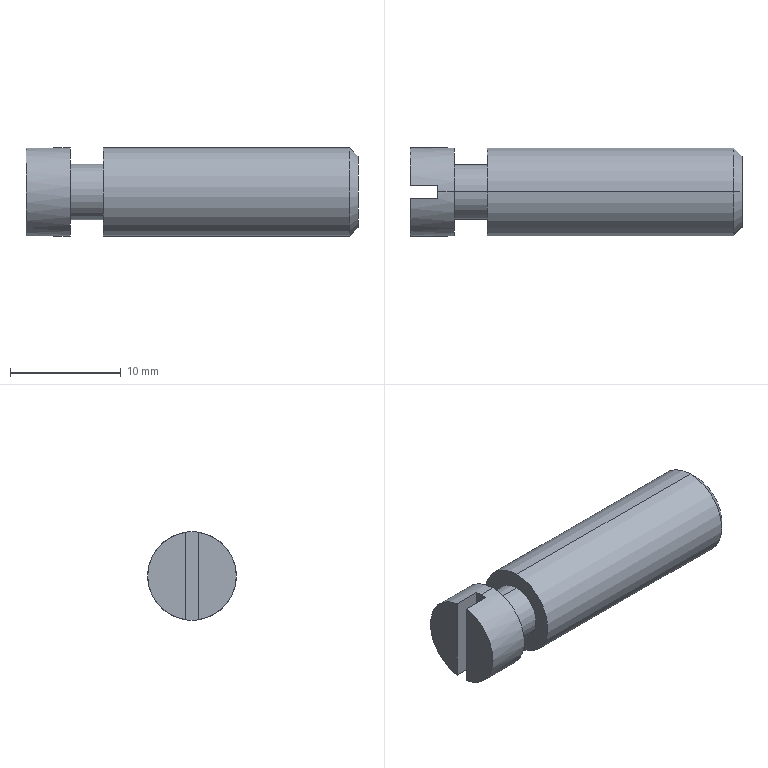Part | STEP file | 0217_Z_SBSP8-30-1 | 1 solid | 16 faces | box 30 x 8 x 8 mm | volume 1385 mm3 | plane 8 | cylinder 6 | cone 2 | commonest cylinder face diameters 8 x4 5 x2
STEP:
#1=CARTESIAN_POINT('',(0.,0.,0.));
#2=DIRECTION('',(0.,0.,1.));
#3=DIRECTION('',(1.,0.,0.));
#4=AXIS2_PLACEMENT_3D('',#1,#2,#3);
#5=CARTESIAN_POINT('',(7.,0.,-4.));
#6=VERTEX_POINT('',#5);
#7=CARTESIAN_POINT('',(7.,0.,4.));
#8=VERTEX_POINT('',#7);
#9=CARTESIAN_POINT('',(7.,0.,0.));
#10=DIRECTION('',(1.,0.,0.));
#11=DIRECTION('',(0.,0.,-1.));
#12=AXIS2_PLACEMENT_3D('',#9,#10,#11);
#13=CIRCLE('',#12,4.);
#14=CARTESIAN_POINT('',(14.617,0.,0.));
#15=DIRECTION('',(1.,0.,0.));
#16=DIRECTION('',(0.,0.,-1.));
#17=AXIS2_PLACEMENT_3D('',#14,#15,#16);
#18=CYLINDRICAL_SURFACE('',#17,4.);
#19=CARTESIAN_POINT('',(0.,-7.617));
#20=DIRECTION('',(1.,0.));
#21=VECTOR('',#20,1.);
#22=LINE('',#19,#21);
#23=(GEOMETRIC_REPRESENTATION_CONTEXT(2)PARAMETRIC_REPRESENTATION_CONTEXT()REPRESENTATION_CONTEXT('',''));
#24=DEFINITIONAL_REPRESENTATION('',(#22),#23);
#25=PCURVE('',#18,#24);
#26=CARTESIAN_POINT('',(7.,4.,0.));
#27=DIRECTION('',(1.,0.,0.));
#28=DIRECTION('',(0.,0.,-1.));
#29=AXIS2_PLACEMENT_3D('',#26,#27,#28);
#30=PLANE('',#29);
#31=CARTESIAN_POINT('',(0.,-4.));
#32=DIRECTION('',(1.,0.));
#33=AXIS2_PLACEMENT_2D('',#31,#32);
#34=CIRCLE('',#33,4.);
#35=(GEOMETRIC_REPRESENTATION_CONTEXT(2)PARAMETRIC_REPRESENTATION_CONTEXT()REPRESENTATION_CONTEXT('',''));
#36=DEFINITIONAL_REPRESENTATION('',(#34),#35);
#37=PCURVE('',#30,#36);
#38=SURFACE_CURVE('',#13,(#25,#37),.PCURVE_S1.);
#39=EDGE_CURVE('',#6,#8,#38,.T.);
#40=ORIENTED_EDGE('',*,*,#39,.T.);
#41=CARTESIAN_POINT('',(29.233,0.,4.));
#42=VERTEX_POINT('',#41);
#43=CARTESIAN_POINT('',(14.617,0.,4.));
#44=DIRECTION('',(1.,0.,0.));
#45=VECTOR('',#44,1.);
#46=LINE('',#43,#45);
#47=CARTESIAN_POINT('',(3.142,0.));
#48=DIRECTION('',(0.,1.));
#49=VECTOR('',#48,1.);
#50=LINE('',#47,#49);
#51=(GEOMETRIC_REPRESENTATION_CONTEXT(2)PARAMETRIC_REPRESENTATION_CONTEXT()REPRESENTATION_CONTEXT('',''));
#52=DEFINITIONAL_REPRESENTATION('',(#50),#51);
#53=PCURVE('',#18,#52);
#54=CARTESIAN_POINT('',(14.617,0.,0.));
#55=DIRECTION('',(1.,0.,0.));
#56=DIRECTION('',(0.,0.,-1.));
#57=AXIS2_PLACEMENT_3D('',#54,#55,#56);
#58=CYLINDRICAL_SURFACE('',#57,4.);
#59=CARTESIAN_POINT('',(3.142,0.));
#60=DIRECTION('',(0.,1.));
#61=VECTOR('',#60,1.);
#62=LINE('',#59,#61);
#63=(GEOMETRIC_REPRESENTATION_CONTEXT(2)PARAMETRIC_REPRESENTATION_CONTEXT()REPRESENTATION_CONTEXT('',''));
#64=DEFINITIONAL_REPRESENTATION('',(#62),#63);
#65=PCURVE('',#58,#64);
#66=SURFACE_CURVE('',#46,(#53,#65),.PCURVE_S1.);
#67=EDGE_CURVE('',#8,#42,#66,.T.);
#68=ORIENTED_EDGE('',*,*,#67,.T.);
#69=CARTESIAN_POINT('',(29.233,0.,-4.));
#70=VERTEX_POINT('',#69);
#71=CARTESIAN_POINT('',(29.233,0.,0.));
#72=DIRECTION('',(-1.,0.,0.));
#73=DIRECTION('',(0.,0.,-1.));
#74=AXIS2_PLACEMENT_3D('',#71,#72,#73);
#75=CIRCLE('',#74,4.);
#76=CARTESIAN_POINT('',(6.283,14.617));
#77=DIRECTION('',(-1.,0.));
#78=VECTOR('',#77,1.);
#79=LINE('',#76,#78);
#80=(GEOMETRIC_REPRESENTATION_CONTEXT(2)PARAMETRIC_REPRESENTATION_CONTEXT()REPRESENTATION_CONTEXT('',''));
#81=DEFINITIONAL_REPRESENTATION('',(#79),#80);
#82=PCURVE('',#18,#81);
#83=CARTESIAN_POINT('',(29.233,0.,0.));
#84=DIRECTION('',(-1.,0.,0.));
#85=DIRECTION('',(0.,0.,1.));
#86=AXIS2_PLACEMENT_3D('',#83,#84,#85);
#87=CONICAL_SURFACE('',#86,4.,0.7854);
#88=CARTESIAN_POINT('',(-3.142,0.));
#89=DIRECTION('',(1.,0.));
#90=VECTOR('',#89,1.);
#91=LINE('',#88,#90);
#92=(GEOMETRIC_REPRESENTATION_CONTEXT(2)PARAMETRIC_REPRESENTATION_CONTEXT()REPRESENTATION_CONTEXT('',''));
#93=DEFINITIONAL_REPRESENTATION('',(#91),#92);
#94=PCURVE('',#87,#93);
#95=SURFACE_CURVE('',#75,(#82,#94),.PCURVE_S1.);
#96=EDGE_CURVE('',#42,#70,#95,.T.);
#97=ORIENTED_EDGE('',*,*,#96,.T.);
#98=CARTESIAN_POINT('',(14.617,0.,-4.));
#99=DIRECTION('',(1.,0.,0.));
#100=VECTOR('',#99,1.);
#101=LINE('',#98,#100);
#102=CARTESIAN_POINT('',(0.,0.));
#103=DIRECTION('',(0.,1.));
#104=VECTOR('',#103,1.);
#105=LINE('',#102,#104);
#106=(GEOMETRIC_REPRESENTATION_CONTEXT(2)PARAMETRIC_REPRESENTATION_CONTEXT()REPRESENTATION_CONTEXT('',''));
#107=DEFINITIONAL_REPRESENTATION('',(#105),#106);
#108=PCURVE('',#18,#107);
#109=CARTESIAN_POINT('',(6.283,0.));
#110=DIRECTION('',(0.,1.));
#111=VECTOR('',#110,1.);
#112=LINE('',#109,#111);
#113=(GEOMETRIC_REPRESENTATION_CONTEXT(2)PARAMETRIC_REPRESENTATION_CONTEXT()REPRESENTATION_CONTEXT('',''));
#114=DEFINITIONAL_REPRESENTATION('',(#112),#113);
#115=PCURVE('',#58,#114);
#116=SURFACE_CURVE('',#101,(#108,#115),.PCURVE_S1.);
#117=EDGE_CURVE('',#6,#70,#116,.T.);
#118=ORIENTED_EDGE('',*,*,#117,.F.);
#119=EDGE_LOOP('',(#40,#68,#97,#118));
#120=FACE_BOUND('',#119,.T.);
#121=ADVANCED_FACE('',(#120),#18,.T.);
#122=CARTESIAN_POINT('',(30.,0.,3.233));
#123=VERTEX_POINT('',#122);
#124=CARTESIAN_POINT('',(30.,0.,-3.233));
#125=VERTEX_POINT('',#124);
#126=CARTESIAN_POINT('',(30.,0.,0.));
#127=DIRECTION('',(-1.,0.,0.));
#128=DIRECTION('',(0.,0.,1.));
#129=AXIS2_PLACEMENT_3D('',#126,#127,#128);
#130=CIRCLE('',#129,3.233);
#131=CARTESIAN_POINT('',(0.,-0.767));
#132=DIRECTION('',(1.,0.));
#133=VECTOR('',#132,1.);
#134=LINE('',#131,#133);
#135=(GEOMETRIC_REPRESENTATION_CONTEXT(2)PARAMETRIC_REPRESENTATION_CONTEXT()REPRESENTATION_CONTEXT('',''));
#136=DEFINITIONAL_REPRESENTATION('',(#134),#135);
#137=PCURVE('',#87,#136);
#138=CARTESIAN_POINT('',(30.,1.617,0.));
#139=DIRECTION('',(1.,0.,0.));
#140=DIRECTION('',(0.,0.,-1.));
#141=AXIS2_PLACEMENT_3D('',#138,#139,#140);
#142=PLANE('',#141);
#143=CARTESIAN_POINT('',(-3.233,-1.617));
#144=CARTESIAN_POINT('',(-3.233,3.983));
#145=CARTESIAN_POINT('',(1.616,1.183));
#146=CARTESIAN_POINT('',(6.466,-1.617));
#147=CARTESIAN_POINT('',(1.616,-4.416));
#148=CARTESIAN_POINT('',(-3.233,-7.216));
#149=CARTESIAN_POINT('',(-3.233,-1.617));
#150=(BOUNDED_CURVE()B_SPLINE_CURVE(2,(#143,#144,#145,#146,#147,#148,#149),.UNSPECIFIED.,.T.,.F.)B_SPLINE_CURVE_WITH_KNOTS((1,2,2,2,2,1),(-2.094,0.,2.094,4.189,6.283,8.378),.UNSPECIFIED.)CURVE()GEOMETRIC_REPRESENTATION_ITEM()RATIONAL_B_SPLINE_CURVE((1.,0.5,1.,0.5,1.,0.5,1.))REPRESENTATION_ITEM(''));
#151=(GEOMETRIC_REPRESENTATION_CONTEXT(2)PARAMETRIC_REPRESENTATION_CONTEXT()REPRESENTATION_CONTEXT('',''));
#152=DEFINITIONAL_REPRESENTATION('',(#150),#151);
#153=PCURVE('',#142,#152);
#154=SURFACE_CURVE('',#130,(#137,#153),.PCURVE_S1.);
#155=EDGE_CURVE('',#123,#125,#154,.T.);
#156=ORIENTED_EDGE('',*,*,#155,.T.);
#157=CARTESIAN_POINT('',(29.233,0.,-4.));
#158=DIRECTION('',(-0.7071,0.,-0.7071));
#159=VECTOR('',#158,1.);
#160=LINE('',#157,#159);
#161=CARTESIAN_POINT('',(3.142,0.));
#162=DIRECTION('',(0.,1.));
#163=VECTOR('',#162,1.);
#164=LINE('',#161,#163);
#165=(GEOMETRIC_REPRESENTATION_CONTEXT(2)PARAMETRIC_REPRESENTATION_CONTEXT()REPRESENTATION_CONTEXT('',''));
#166=DEFINITIONAL_REPRESENTATION('',(#164),#165);
#167=PCURVE('',#87,#166);
#168=CARTESIAN_POINT('',(29.233,0.,0.));
#169=DIRECTION('',(-1.,0.,0.));
#170=DIRECTION('',(0.,0.,1.));
#171=AXIS2_PLACEMENT_3D('',#168,#169,#170);
#172=CONICAL_SURFACE('',#171,4.,0.7854);
#173=CARTESIAN_POINT('',(3.142,0.));
#174=DIRECTION('',(0.,1.));
#175=VECTOR('',#174,1.);
#176=LINE('',#173,#175);
#177=(GEOMETRIC_REPRESENTATION_CONTEXT(2)PARAMETRIC_REPRESENTATION_CONTEXT()REPRESENTATION_CONTEXT('',''));
#178=DEFINITIONAL_REPRESENTATION('',(#176),#177);
#179=PCURVE('',#172,#178);
#180=SURFACE_CURVE('',#160,(#167,#179),.PCURVE_S1.);
#181=EDGE_CURVE('',#125,#70,#180,.T.);
#182=ORIENTED_EDGE('',*,*,#181,.T.);
#183=ORIENTED_EDGE('',*,*,#96,.F.);
#184=CARTESIAN_POINT('',(29.233,0.,4.));
#185=DIRECTION('',(-0.7071,0.,0.7071));
#186=VECTOR('',#185,1.);
#187=LINE('',#184,#186);
#188=CARTESIAN_POINT('',(0.,0.));
#189=DIRECTION('',(0.,1.));
#190=VECTOR('',#189,1.);
#191=LINE('',#188,#190);
#192=(GEOMETRIC_REPRESENTATION_CONTEXT(2)PARAMETRIC_REPRESENTATION_CONTEXT()REPRESENTATION_CONTEXT('',''));
#193=DEFINITIONAL_REPRESENTATION('',(#191),#192);
#194=PCURVE('',#87,#193);
#195=CARTESIAN_POINT('',(6.283,0.));
#196=DIRECTION('',(0.,1.));
#197=VECTOR('',#196,1.);
#198=LINE('',#195,#197);
#199=(GEOMETRIC_REPRESENTATION_CONTEXT(2)PARAMETRIC_REPRESENTATION_CONTEXT()REPRESENTATION_CONTEXT('',''));
#200=DEFINITIONAL_REPRESENTATION('',(#198),#199);
#201=PCURVE('',#172,#200);
#202=SURFACE_CURVE('',#187,(#194,#201),.PCURVE_S1.);
#203=EDGE_CURVE('',#123,#42,#202,.T.);
#204=ORIENTED_EDGE('',*,*,#203,.F.);
#205=EDGE_LOOP('',(#156,#182,#183,#204));
#206=FACE_BOUND('',#205,.T.);
#207=ADVANCED_FACE('',(#206),#87,.T.);
#208=CARTESIAN_POINT('',(4.,0.,-2.5));
#209=VERTEX_POINT('',#208);
#210=CARTESIAN_POINT('',(4.,0.,2.5));
#211=VERTEX_POINT('',#210);
#212=CARTESIAN_POINT('',(4.,0.,0.));
#213=DIRECTION('',(1.,0.,0.));
#214=DIRECTION('',(0.,0.,-1.));
#215=AXIS2_PLACEMENT_3D('',#212,#213,#214);
#216=CIRCLE('',#215,2.5);
#217=CARTESIAN_POINT('',(5.5,0.,0.));
#218=DIRECTION('',(1.,0.,0.));
#219=DIRECTION('',(0.,0.,-1.));
#220=AXIS2_PLACEMENT_3D('',#217,#218,#219);
#221=CYLINDRICAL_SURFACE('',#220,2.5);
#222=CARTESIAN_POINT('',(0.,-1.5));
#223=DIRECTION('',(1.,0.));
#224=VECTOR('',#223,1.);
#225=LINE('',#222,#224);
#226=(GEOMETRIC_REPRESENTATION_CONTEXT(2)PARAMETRIC_REPRESENTATION_CONTEXT()REPRESENTATION_CONTEXT('',''));
#227=DEFINITIONAL_REPRESENTATION('',(#225),#226);
#228=PCURVE('',#221,#227);
#229=CARTESIAN_POINT('',(4.,4.,0.));
#230=DIRECTION('',(-1.,0.,0.));
#231=DIRECTION('',(0.,0.,1.));
#232=AXIS2_PLACEMENT_3D('',#229,#230,#231);
#233=PLANE('',#232);
#234=CARTESIAN_POINT('',(-2.5,-4.));
#235=CARTESIAN_POINT('',(-2.5,0.3301));
#236=CARTESIAN_POINT('',(1.25,-1.835));
#237=CARTESIAN_POINT('',(5.,-4.));
#238=CARTESIAN_POINT('',(1.25,-6.165));
#239=CARTESIAN_POINT('',(-2.5,-8.33));
#240=CARTESIAN_POINT('',(-2.5,-4.));
#241=(BOUNDED_CURVE()B_SPLINE_CURVE(2,(#234,#235,#236,#237,#238,#239,#240),.UNSPECIFIED.,.T.,.F.)B_SPLINE_CURVE_WITH_KNOTS((1,2,2,2,2,1),(-2.094,0.,2.094,4.189,6.283,8.378),.UNSPECIFIED.)CURVE()GEOMETRIC_REPRESENTATION_ITEM()RATIONAL_B_SPLINE_CURVE((1.,0.5,1.,0.5,1.,0.5,1.))REPRESENTATION_ITEM(''));
#242=(GEOMETRIC_REPRESENTATION_CONTEXT(2)PARAMETRIC_REPRESENTATION_CONTEXT()REPRESENTATION_CONTEXT('',''));
#243=DEFINITIONAL_REPRESENTATION('',(#241),#242);
#244=PCURVE('',#233,#243);
#245=SURFACE_CURVE('',#216,(#228,#244),.PCURVE_S1.);
#246=EDGE_CURVE('',#209,#211,#245,.T.);
#247=ORIENTED_EDGE('',*,*,#246,.T.);
#248=CARTESIAN_POINT('',(7.,0.,2.5));
#249=VERTEX_POINT('',#248);
#250=CARTESIAN_POINT('',(5.5,0.,2.5));
#251=DIRECTION('',(1.,0.,0.));
#252=VECTOR('',#251,1.);
#253=LINE('',#250,#252);
#254=CARTESIAN_POINT('',(3.142,0.));
#255=DIRECTION('',(0.,1.));
#256=VECTOR('',#255,1.);
#257=LINE('',#254,#256);
#258=(GEOMETRIC_REPRESENTATION_CONTEXT(2)PARAMETRIC_REPRESENTATION_CONTEXT()REPRESENTATION_CONTEXT('',''));
#259=DEFINITIONAL_REPRESENTATION('',(#257),#258);
#260=PCURVE('',#221,#259);
#261=CARTESIAN_POINT('',(5.5,0.,0.));
#262=DIRECTION('',(1.,0.,0.));
#263=DIRECTION('',(0.,0.,-1.));
#264=AXIS2_PLACEMENT_3D('',#261,#262,#263);
#265=CYLINDRICAL_SURFACE('',#264,2.5);
#266=CARTESIAN_POINT('',(3.142,0.));
#267=DIRECTION('',(0.,1.));
#268=VECTOR('',#267,1.);
#269=LINE('',#266,#268);
#270=(GEOMETRIC_REPRESENTATION_CONTEXT(2)PARAMETRIC_REPRESENTATION_CONTEXT()REPRESENTATION_CONTEXT('',''));
#271=DEFINITIONAL_REPRESENTATION('',(#269),#270);
#272=PCURVE('',#265,#271);
#273=SURFACE_CURVE('',#253,(#260,#272),.PCURVE_S1.);
#274=EDGE_CURVE('',#211,#249,#273,.T.);
#275=ORIENTED_EDGE('',*,*,#274,.T.);
#276=CARTESIAN_POINT('',(7.,0.,-2.5));
#277=VERTEX_POINT('',#276);
#278=CARTESIAN_POINT('',(7.,0.,0.));
#279=DIRECTION('',(-1.,0.,0.));
#280=DIRECTION('',(0.,0.,-1.));
#281=AXIS2_PLACEMENT_3D('',#278,#279,#280);
#282=CIRCLE('',#281,2.5);
#283=CARTESIAN_POINT('',(6.283,1.5));
#284=DIRECTION('',(-1.,0.));
#285=VECTOR('',#284,1.);
#286=LINE('',#283,#285);
#287=(GEOMETRIC_REPRESENTATION_CONTEXT(2)PARAMETRIC_REPRESENTATION_CONTEXT()REPRESENTATION_CONTEXT('',''));
#288=DEFINITIONAL_REPRESENTATION('',(#286),#287);
#289=PCURVE('',#221,#288);
#290=CARTESIAN_POINT('',(2.5,-4.));
#291=CARTESIAN_POINT('',(2.5,-8.33));
#292=CARTESIAN_POINT('',(-1.25,-6.165));
#293=CARTESIAN_POINT('',(-5.,-4.));
#294=CARTESIAN_POINT('',(-1.25,-1.835));
#295=CARTESIAN_POINT('',(2.5,0.3301));
#296=CARTESIAN_POINT('',(2.5,-4.));
#297=(BOUNDED_CURVE()B_SPLINE_CURVE(2,(#290,#291,#292,#293,#294,#295,#296),.UNSPECIFIED.,.T.,.F.)B_SPLINE_CURVE_WITH_KNOTS((1,2,2,2,2,1),(-2.094,0.,2.094,4.189,6.283,8.378),.UNSPECIFIED.)CURVE()GEOMETRIC_REPRESENTATION_ITEM()RATIONAL_B_SPLINE_CURVE((1.,0.5,1.,0.5,1.,0.5,1.))REPRESENTATION_ITEM(''));
#298=(GEOMETRIC_REPRESENTATION_CONTEXT(2)PARAMETRIC_REPRESENTATION_CONTEXT()REPRESENTATION_CONTEXT('',''));
#299=DEFINITIONAL_REPRESENTATION('',(#297),#298);
#300=PCURVE('',#30,#299);
#301=SURFACE_CURVE('',#282,(#289,#300),.PCURVE_S1.);
#302=EDGE_CURVE('',#249,#277,#301,.T.);
#303=ORIENTED_EDGE('',*,*,#302,.T.);
#304=CARTESIAN_POINT('',(5.5,0.,-2.5));
#305=DIRECTION('',(1.,0.,0.));
#306=VECTOR('',#305,1.);
#307=LINE('',#304,#306);
#308=CARTESIAN_POINT('',(0.,0.));
#309=DIRECTION('',(0.,1.));
#310=VECTOR('',#309,1.);
#311=LINE('',#308,#310);
#312=(GEOMETRIC_REPRESENTATION_CONTEXT(2)PARAMETRIC_REPRESENTATION_CONTEXT()REPRESENTATION_CONTEXT('',''));
#313=DEFINITIONAL_REPRESENTATION('',(#311),#312);
#314=PCURVE('',#221,#313);
#315=CARTESIAN_POINT('',(6.283,0.));
#316=DIRECTION('',(0.,1.));
#317=VECTOR('',#316,1.);
#318=LINE('',#315,#317);
#319=(GEOMETRIC_REPRESENTATION_CONTEXT(2)PARAMETRIC_REPRESENTATION_CONTEXT()REPRESENTATION_CONTEXT('',''));
#320=DEFINITIONAL_REPRESENTATION('',(#318),#319);
#321=PCURVE('',#265,#320);
#322=SURFACE_CURVE('',#307,(#314,#321),.PCURVE_S1.);
#323=EDGE_CURVE('',#209,#277,#322,.T.);
#324=ORIENTED_EDGE('',*,*,#323,.F.);
#325=EDGE_LOOP('',(#247,#275,#303,#324));
#326=FACE_BOUND('',#325,.T.);
#327=ADVANCED_FACE('',(#326),#221,.T.);
#328=CARTESIAN_POINT('',(2.5,0.6,3.955));
#329=VERTEX_POINT('',#328);
#330=CARTESIAN_POINT('',(2.5,0.,4.));
#331=VERTEX_POINT('',#330);
#332=CARTESIAN_POINT('',(2.5,0.,0.));
#333=DIRECTION('',(1.,0.,0.));
#334=DIRECTION('',(0.,0.,-1.));
#335=AXIS2_PLACEMENT_3D('',#332,#333,#334);
#336=CIRCLE('',#335,4.);
#337=CARTESIAN_POINT('',(14.617,0.,0.));
#338=DIRECTION('',(1.,0.,0.));
#339=DIRECTION('',(0.,0.,-1.));
#340=AXIS2_PLACEMENT_3D('',#337,#338,#339);
#341=CYLINDRICAL_SURFACE('',#340,4.);
#342=CARTESIAN_POINT('',(0.,-12.117));
#343=DIRECTION('',(1.,0.));
#344=VECTOR('',#343,1.);
#345=LINE('',#342,#344);
#346=(GEOMETRIC_REPRESENTATION_CONTEXT(2)PARAMETRIC_REPRESENTATION_CONTEXT()REPRESENTATION_CONTEXT('',''));
#347=DEFINITIONAL_REPRESENTATION('',(#345),#346);
#348=PCURVE('',#341,#347);
#349=CARTESIAN_POINT('',(2.5,-0.6,4.));
#350=DIRECTION('',(1.,0.,0.));
#351=DIRECTION('',(0.,0.,-1.));
#352=AXIS2_PLACEMENT_3D('',#349,#350,#351);
#353=PLANE('',#352);
#354=CARTESIAN_POINT('',(4.,0.6));
#355=DIRECTION('',(1.,0.));
#356=AXIS2_PLACEMENT_2D('',#354,#355);
#357=CIRCLE('',#356,4.);
#358=(GEOMETRIC_REPRESENTATION_CONTEXT(2)PARAMETRIC_REPRESENTATION_CONTEXT()REPRESENTATION_CONTEXT('',''));
#359=DEFINITIONAL_REPRESENTATION('',(#357),#358);
#360=PCURVE('',#353,#359);
#361=SURFACE_CURVE('',#336,(#348,#360),.PCURVE_S1.);
#362=EDGE_CURVE('',#329,#331,#361,.T.);
#363=ORIENTED_EDGE('',*,*,#362,.T.);
#364=CARTESIAN_POINT('',(4.,0.,4.));
#365=VERTEX_POINT('',#364);
#366=CARTESIAN_POINT('',(14.617,0.,4.));
#367=DIRECTION('',(1.,0.,0.));
#368=VECTOR('',#367,1.);
#369=LINE('',#366,#368);
#370=CARTESIAN_POINT('',(3.142,0.));
#371=DIRECTION('',(0.,1.));
#372=VECTOR('',#371,1.);
#373=LINE('',#370,#372);
#374=(GEOMETRIC_REPRESENTATION_CONTEXT(2)PARAMETRIC_REPRESENTATION_CONTEXT()REPRESENTATION_CONTEXT('',''));
#375=DEFINITIONAL_REPRESENTATION('',(#373),#374);
#376=PCURVE('',#341,#375);
#377=CARTESIAN_POINT('',(14.617,0.,0.));
#378=DIRECTION('',(1.,0.,0.));
#379=DIRECTION('',(0.,0.,-1.));
#380=AXIS2_PLACEMENT_3D('',#377,#378,#379);
#381=CYLINDRICAL_SURFACE('',#380,4.);
#382=CARTESIAN_POINT('',(3.142,0.));
#383=DIRECTION('',(0.,1.));
#384=VECTOR('',#383,1.);
#385=LINE('',#382,#384);
#386=(GEOMETRIC_REPRESENTATION_CONTEXT(2)PARAMETRIC_REPRESENTATION_CONTEXT()REPRESENTATION_CONTEXT('',''));
#387=DEFINITIONAL_REPRESENTATION('',(#385),#386);
#388=PCURVE('',#381,#387);
#389=SURFACE_CURVE('',#369,(#376,#388),.PCURVE_S1.);
#390=EDGE_CURVE('',#331,#365,#389,.T.);
#391=ORIENTED_EDGE('',*,*,#390,.T.);
#392=CARTESIAN_POINT('',(4.,0.,-4.));
#393=VERTEX_POINT('',#392);
#394=CARTESIAN_POINT('',(4.,0.,0.));
#395=DIRECTION('',(-1.,0.,0.));
#396=DIRECTION('',(0.,0.,-1.));
#397=AXIS2_PLACEMENT_3D('',#394,#395,#396);
#398=CIRCLE('',#397,4.);
#399=CARTESIAN_POINT('',(6.283,-10.617));
#400=DIRECTION('',(-1.,0.));
#401=VECTOR('',#400,1.);
#402=LINE('',#399,#401);
#403=(GEOMETRIC_REPRESENTATION_CONTEXT(2)PARAMETRIC_REPRESENTATION_CONTEXT()REPRESENTATION_CONTEXT('',''));
#404=DEFINITIONAL_REPRESENTATION('',(#402),#403);
#405=PCURVE('',#341,#404);
#406=CARTESIAN_POINT('',(0.,-4.));
#407=DIRECTION('',(-1.,0.));
#408=AXIS2_PLACEMENT_2D('',#406,#407);
#409=CIRCLE('',#408,4.);
#410=(GEOMETRIC_REPRESENTATION_CONTEXT(2)PARAMETRIC_REPRESENTATION_CONTEXT()REPRESENTATION_CONTEXT('',''));
#411=DEFINITIONAL_REPRESENTATION('',(#409),#410);
#412=PCURVE('',#233,#411);
#413=SURFACE_CURVE('',#398,(#405,#412),.PCURVE_S1.);
#414=EDGE_CURVE('',#365,#393,#413,.T.);
#415=ORIENTED_EDGE('',*,*,#414,.T.);
#416=CARTESIAN_POINT('',(2.5,0.,-4.));
#417=VERTEX_POINT('',#416);
#418=CARTESIAN_POINT('',(14.617,0.,-4.));
#419=DIRECTION('',(1.,0.,0.));
#420=VECTOR('',#419,1.);
#421=LINE('',#418,#420);
#422=CARTESIAN_POINT('',(0.,0.));
#423=DIRECTION('',(0.,1.));
#424=VECTOR('',#423,1.);
#425=LINE('',#422,#424);
#426=(GEOMETRIC_REPRESENTATION_CONTEXT(2)PARAMETRIC_REPRESENTATION_CONTEXT()REPRESENTATION_CONTEXT('',''));
#427=DEFINITIONAL_REPRESENTATION('',(#425),#426);
#428=PCURVE('',#341,#427);
#429=CARTESIAN_POINT('',(6.283,0.));
#430=DIRECTION('',(0.,1.));
#431=VECTOR('',#430,1.);
#432=LINE('',#429,#431);
#433=(GEOMETRIC_REPRESENTATION_CONTEXT(2)PARAMETRIC_REPRESENTATION_CONTEXT()REPRESENTATION_CONTEXT('',''));
#434=DEFINITIONAL_REPRESENTATION('',(#432),#433);
#435=PCURVE('',#381,#434);
#436=SURFACE_CURVE('',#421,(#428,#435),.PCURVE_S1.);
#437=EDGE_CURVE('',#417,#393,#436,.T.);
#438=ORIENTED_EDGE('',*,*,#437,.F.);
#439=CARTESIAN_POINT('',(2.5,0.6,-3.955));
#440=VERTEX_POINT('',#439);
#441=CARTESIAN_POINT('',(2.5,0.,0.));
#442=DIRECTION('',(1.,0.,0.));
#443=DIRECTION('',(0.,0.,-1.));
#444=AXIS2_PLACEMENT_3D('',#441,#442,#443);
#445=CIRCLE('',#444,4.);
#446=CARTESIAN_POINT('',(0.,-12.117));
#447=DIRECTION('',(1.,0.));
#448=VECTOR('',#447,1.);
#449=LINE('',#446,#448);
#450=(GEOMETRIC_REPRESENTATION_CONTEXT(2)PARAMETRIC_REPRESENTATION_CONTEXT()REPRESENTATION_CONTEXT('',''));
#451=DEFINITIONAL_REPRESENTATION('',(#449),#450);
#452=PCURVE('',#341,#451);
#453=CARTESIAN_POINT('',(4.,0.6));
#454=DIRECTION('',(1.,0.));
#455=AXIS2_PLACEMENT_2D('',#453,#454);
#456=CIRCLE('',#455,4.);
#457=(GEOMETRIC_REPRESENTATION_CONTEXT(2)PARAMETRIC_REPRESENTATION_CONTEXT()REPRESENTATION_CONTEXT('',''));
#458=DEFINITIONAL_REPRESENTATION('',(#456),#457);
#459=PCURVE('',#353,#458);
#460=SURFACE_CURVE('',#445,(#452,#459),.PCURVE_S1.);
#461=EDGE_CURVE('',#417,#440,#460,.T.);
#462=ORIENTED_EDGE('',*,*,#461,.T.);
#463=CARTESIAN_POINT('',(0.,0.6,-3.955));
#464=VERTEX_POINT('',#463);
#465=CARTESIAN_POINT('',(14.617,0.6,-3.955));
#466=DIRECTION('',(-1.,0.,0.));
#467=VECTOR('',#466,1.);
#468=LINE('',#465,#467);
#469=CARTESIAN_POINT('',(0.1506,0.));
#470=DIRECTION('',(0.,-1.));
#471=VECTOR('',#470,1.);
#472=LINE('',#469,#471);
#473=(GEOMETRIC_REPRESENTATION_CONTEXT(2)PARAMETRIC_REPRESENTATION_CONTEXT()REPRESENTATION_CONTEXT('',''));
#474=DEFINITIONAL_REPRESENTATION('',(#472),#473);
#475=PCURVE('',#341,#474);
#476=CARTESIAN_POINT('',(2.5,0.6,4.));
#477=DIRECTION('',(0.,1.,0.));
#478=DIRECTION('',(0.,0.,1.));
#479=AXIS2_PLACEMENT_3D('',#476,#477,#478);
#480=PLANE('',#479);
#481=CARTESIAN_POINT('',(-7.955,12.117));
#482=DIRECTION('',(0.,-1.));
#483=VECTOR('',#482,1.);
#484=LINE('',#481,#483);
#485=(GEOMETRIC_REPRESENTATION_CONTEXT(2)PARAMETRIC_REPRESENTATION_CONTEXT()REPRESENTATION_CONTEXT('',''));
#486=DEFINITIONAL_REPRESENTATION('',(#484),#485);
#487=PCURVE('',#480,#486);
#488=SURFACE_CURVE('',#468,(#475,#487),.PCURVE_S1.);
#489=EDGE_CURVE('',#440,#464,#488,.T.);
#490=ORIENTED_EDGE('',*,*,#489,.T.);
#491=CARTESIAN_POINT('',(0.,0.6,3.955));
#492=VERTEX_POINT('',#491);
#493=CARTESIAN_POINT('',(0.,0.,0.));
#494=DIRECTION('',(1.,0.,0.));
#495=DIRECTION('',(0.,0.,-1.));
#496=AXIS2_PLACEMENT_3D('',#493,#494,#495);
#497=CIRCLE('',#496,4.);
#498=CARTESIAN_POINT('',(0.,-14.617));
#499=DIRECTION('',(1.,0.));
#500=VECTOR('',#499,1.);
#501=LINE('',#498,#500);
#502=(GEOMETRIC_REPRESENTATION_CONTEXT(2)PARAMETRIC_REPRESENTATION_CONTEXT()REPRESENTATION_CONTEXT('',''));
#503=DEFINITIONAL_REPRESENTATION('',(#501),#502);
#504=PCURVE('',#341,#503);
#505=CARTESIAN_POINT('',(0.,2.,0.));
#506=DIRECTION('',(-1.,0.,0.));
#507=DIRECTION('',(0.,0.,1.));
#508=AXIS2_PLACEMENT_3D('',#505,#506,#507);
#509=PLANE('',#508);
#510=CARTESIAN_POINT('',(-4.,-2.));
#511=CARTESIAN_POINT('',(-4.,4.928));
#512=CARTESIAN_POINT('',(2.,1.464));
#513=CARTESIAN_POINT('',(8.,-2.));
#514=CARTESIAN_POINT('',(2.,-5.464));
#515=CARTESIAN_POINT('',(-4.,-8.928));
#516=CARTESIAN_POINT('',(-4.,-2.));
#517=(BOUNDED_CURVE()B_SPLINE_CURVE(2,(#510,#511,#512,#513,#514,#515,#516),.UNSPECIFIED.,.T.,.F.)B_SPLINE_CURVE_WITH_KNOTS((1,2,2,2,2,1),(-2.094,0.,2.094,4.189,6.283,8.378),.UNSPECIFIED.)CURVE()GEOMETRIC_REPRESENTATION_ITEM()RATIONAL_B_SPLINE_CURVE((1.,0.5,1.,0.5,1.,0.5,1.))REPRESENTATION_ITEM(''));
#518=(GEOMETRIC_REPRESENTATION_CONTEXT(2)PARAMETRIC_REPRESENTATION_CONTEXT()REPRESENTATION_CONTEXT('',''));
#519=DEFINITIONAL_REPRESENTATION('',(#517),#518);
#520=PCURVE('',#509,#519);
#521=SURFACE_CURVE('',#497,(#504,#520),.PCURVE_S1.);
#522=EDGE_CURVE('',#464,#492,#521,.T.);
#523=ORIENTED_EDGE('',*,*,#522,.T.);
#524=CARTESIAN_POINT('',(14.617,0.6,3.955));
#525=DIRECTION('',(1.,0.,0.));
#526=VECTOR('',#525,1.);
#527=LINE('',#524,#526);
#528=CARTESIAN_POINT('',(2.991,0.));
#529=DIRECTION('',(0.,1.));
#530=VECTOR('',#529,1.);
#531=LINE('',#528,#530);
#532=(GEOMETRIC_REPRESENTATION_CONTEXT(2)PARAMETRIC_REPRESENTATION_CONTEXT()REPRESENTATION_CONTEXT('',''));
#533=DEFINITIONAL_REPRESENTATION('',(#531),#532);
#534=PCURVE('',#341,#533);
#535=CARTESIAN_POINT('',(-0.04526,12.117));
#536=DIRECTION('',(0.,1.));
#537=VECTOR('',#536,1.);
#538=LINE('',#535,#537);
#539=(GEOMETRIC_REPRESENTATION_CONTEXT(2)PARAMETRIC_REPRESENTATION_CONTEXT()REPRESENTATION_CONTEXT('',''));
#540=DEFINITIONAL_REPRESENTATION('',(#538),#539);
#541=PCURVE('',#480,#540);
#542=SURFACE_CURVE('',#527,(#534,#541),.PCURVE_S1.);
#543=EDGE_CURVE('',#492,#329,#542,.T.);
#544=ORIENTED_EDGE('',*,*,#543,.T.);
#545=EDGE_LOOP('',(#363,#391,#415,#438,#462,#490,#523,#544));
#546=FACE_BOUND('',#545,.T.);
#547=ADVANCED_FACE('',(#546),#341,.T.);
#548=ORIENTED_EDGE('',*,*,#67,.F.);
#549=CARTESIAN_POINT('',(7.,0.,0.));
#550=DIRECTION('',(1.,0.,0.));
#551=DIRECTION('',(0.,0.,-1.));
#552=AXIS2_PLACEMENT_3D('',#549,#550,#551);
#553=CIRCLE('',#552,4.);
#554=CARTESIAN_POINT('',(0.,-7.617));
#555=DIRECTION('',(1.,0.));
#556=VECTOR('',#555,1.);
#557=LINE('',#554,#556);
#558=(GEOMETRIC_REPRESENTATION_CONTEXT(2)PARAMETRIC_REPRESENTATION_CONTEXT()REPRESENTATION_CONTEXT('',''));
#559=DEFINITIONAL_REPRESENTATION('',(#557),#558);
#560=PCURVE('',#58,#559);
#561=CARTESIAN_POINT('',(0.,-4.));
#562=DIRECTION('',(1.,0.));
#563=AXIS2_PLACEMENT_2D('',#561,#562);
#564=CIRCLE('',#563,4.);
#565=(GEOMETRIC_REPRESENTATION_CONTEXT(2)PARAMETRIC_REPRESENTATION_CONTEXT()REPRESENTATION_CONTEXT('',''));
#566=DEFINITIONAL_REPRESENTATION('',(#564),#565);
#567=PCURVE('',#30,#566);
#568=SURFACE_CURVE('',#553,(#560,#567),.PCURVE_S1.);
#569=EDGE_CURVE('',#8,#6,#568,.T.);
#570=ORIENTED_EDGE('',*,*,#569,.T.);
#571=ORIENTED_EDGE('',*,*,#117,.T.);
#572=CARTESIAN_POINT('',(29.233,0.,0.));
#573=DIRECTION('',(-1.,0.,0.));
#574=DIRECTION('',(0.,0.,-1.));
#575=AXIS2_PLACEMENT_3D('',#572,#573,#574);
#576=CIRCLE('',#575,4.);
#577=CARTESIAN_POINT('',(6.283,14.617));
#578=DIRECTION('',(-1.,0.));
#579=VECTOR('',#578,1.);
#580=LINE('',#577,#579);
#581=(GEOMETRIC_REPRESENTATION_CONTEXT(2)PARAMETRIC_REPRESENTATION_CONTEXT()REPRESENTATION_CONTEXT('',''));
#582=DEFINITIONAL_REPRESENTATION('',(#580),#581);
#583=PCURVE('',#58,#582);
#584=CARTESIAN_POINT('',(3.142,0.));
#585=DIRECTION('',(1.,0.));
#586=VECTOR('',#585,1.);
#587=LINE('',#584,#586);
#588=(GEOMETRIC_REPRESENTATION_CONTEXT(2)PARAMETRIC_REPRESENTATION_CONTEXT()REPRESENTATION_CONTEXT('',''));
#589=DEFINITIONAL_REPRESENTATION('',(#587),#588);
#590=PCURVE('',#172,#589);
#591=SURFACE_CURVE('',#576,(#583,#590),.PCURVE_S1.);
#592=EDGE_CURVE('',#70,#42,#591,.T.);
#593=ORIENTED_EDGE('',*,*,#592,.T.);
#594=EDGE_LOOP('',(#548,#570,#571,#593));
#595=FACE_BOUND('',#594,.T.);
#596=ADVANCED_FACE('',(#595),#58,.T.);
#597=CARTESIAN_POINT('',(7.,0.,0.));
#598=DIRECTION('',(-1.,0.,0.));
#599=DIRECTION('',(0.,0.,-1.));
#600=AXIS2_PLACEMENT_3D('',#597,#598,#599);
#601=CIRCLE('',#600,2.5);
#602=CARTESIAN_POINT('',(2.5,-4.));
#603=CARTESIAN_POINT('',(2.5,-8.33));
#604=CARTESIAN_POINT('',(-1.25,-6.165));
#605=CARTESIAN_POINT('',(-5.,-4.));
#606=CARTESIAN_POINT('',(-1.25,-1.835));
#607=CARTESIAN_POINT('',(2.5,0.3301));
#608=CARTESIAN_POINT('',(2.5,-4.));
#609=(BOUNDED_CURVE()B_SPLINE_CURVE(2,(#602,#603,#604,#605,#606,#607,#608),.UNSPECIFIED.,.T.,.F.)B_SPLINE_CURVE_WITH_KNOTS((1,2,2,2,2,1),(-2.094,0.,2.094,4.189,6.283,8.378),.UNSPECIFIED.)CURVE()GEOMETRIC_REPRESENTATION_ITEM()RATIONAL_B_SPLINE_CURVE((1.,0.5,1.,0.5,1.,0.5,1.))REPRESENTATION_ITEM(''));
#610=(GEOMETRIC_REPRESENTATION_CONTEXT(2)PARAMETRIC_REPRESENTATION_CONTEXT()REPRESENTATION_CONTEXT('',''));
#611=DEFINITIONAL_REPRESENTATION('',(#609),#610);
#612=PCURVE('',#30,#611);
#613=CARTESIAN_POINT('',(6.283,1.5));
#614=DIRECTION('',(-1.,0.));
#615=VECTOR('',#614,1.);
#616=LINE('',#613,#615);
#617=(GEOMETRIC_REPRESENTATION_CONTEXT(2)PARAMETRIC_REPRESENTATION_CONTEXT()REPRESENTATION_CONTEXT('',''));
#618=DEFINITIONAL_REPRESENTATION('',(#616),#617);
#619=PCURVE('',#265,#618);
#620=SURFACE_CURVE('',#601,(#612,#619),.PCURVE_S1.);
#621=EDGE_CURVE('',#277,#249,#620,.T.);
#622=ORIENTED_EDGE('',*,*,#621,.F.);
#623=ORIENTED_EDGE('',*,*,#302,.F.);
#624=EDGE_LOOP('',(#622,#623));
#625=FACE_BOUND('',#624,.T.);
#626=ORIENTED_EDGE('',*,*,#39,.F.);
#627=ORIENTED_EDGE('',*,*,#569,.F.);
#628=EDGE_LOOP('',(#626,#627));
#629=FACE_BOUND('',#628,.T.);
#630=ADVANCED_FACE('',(#625,#629),#30,.F.);
#631=ORIENTED_EDGE('',*,*,#181,.F.);
#632=CARTESIAN_POINT('',(30.,0.,0.));
#633=DIRECTION('',(-1.,0.,0.));
#634=DIRECTION('',(0.,0.,1.));
#635=AXIS2_PLACEMENT_3D('',#632,#633,#634);
#636=CIRCLE('',#635,3.233);
#637=CARTESIAN_POINT('',(0.,-0.767));
#638=DIRECTION('',(1.,0.));
#639=VECTOR('',#638,1.);
#640=LINE('',#637,#639);
#641=(GEOMETRIC_REPRESENTATION_CONTEXT(2)PARAMETRIC_REPRESENTATION_CONTEXT()REPRESENTATION_CONTEXT('',''));
#642=DEFINITIONAL_REPRESENTATION('',(#640),#641);
#643=PCURVE('',#172,#642);
#644=CARTESIAN_POINT('',(-3.233,-1.617));
#645=CARTESIAN_POINT('',(-3.233,3.983));
#646=CARTESIAN_POINT('',(1.616,1.183));
#647=CARTESIAN_POINT('',(6.466,-1.617));
#648=CARTESIAN_POINT('',(1.616,-4.416));
#649=CARTESIAN_POINT('',(-3.233,-7.216));
#650=CARTESIAN_POINT('',(-3.233,-1.617));
#651=(BOUNDED_CURVE()B_SPLINE_CURVE(2,(#644,#645,#646,#647,#648,#649,#650),.UNSPECIFIED.,.T.,.F.)B_SPLINE_CURVE_WITH_KNOTS((1,2,2,2,2,1),(-2.094,0.,2.094,4.189,6.283,8.378),.UNSPECIFIED.)CURVE()GEOMETRIC_REPRESENTATION_ITEM()RATIONAL_B_SPLINE_CURVE((1.,0.5,1.,0.5,1.,0.5,1.))REPRESENTATION_ITEM(''));
#652=(GEOMETRIC_REPRESENTATION_CONTEXT(2)PARAMETRIC_REPRESENTATION_CONTEXT()REPRESENTATION_CONTEXT('',''));
#653=DEFINITIONAL_REPRESENTATION('',(#651),#652);
#654=PCURVE('',#142,#653);
#655=SURFACE_CURVE('',#636,(#643,#654),.PCURVE_S1.);
#656=EDGE_CURVE('',#125,#123,#655,.T.);
#657=ORIENTED_EDGE('',*,*,#656,.T.);
#658=ORIENTED_EDGE('',*,*,#203,.T.);
#659=ORIENTED_EDGE('',*,*,#592,.F.);
#660=EDGE_LOOP('',(#631,#657,#658,#659));
#661=FACE_BOUND('',#660,.T.);
#662=ADVANCED_FACE('',(#661),#172,.T.);
#663=ORIENTED_EDGE('',*,*,#274,.F.);
#664=CARTESIAN_POINT('',(4.,0.,0.));
#665=DIRECTION('',(1.,0.,0.));
#666=DIRECTION('',(0.,0.,-1.));
#667=AXIS2_PLACEMENT_3D('',#664,#665,#666);
#668=CIRCLE('',#667,2.5);
#669=CARTESIAN_POINT('',(0.,-1.5));
#670=DIRECTION('',(1.,0.));
#671=VECTOR('',#670,1.);
#672=LINE('',#669,#671);
#673=(GEOMETRIC_REPRESENTATION_CONTEXT(2)PARAMETRIC_REPRESENTATION_CONTEXT()REPRESENTATION_CONTEXT('',''));
#674=DEFINITIONAL_REPRESENTATION('',(#672),#673);
#675=PCURVE('',#265,#674);
#676=CARTESIAN_POINT('',(-2.5,-4.));
#677=CARTESIAN_POINT('',(-2.5,0.3301));
#678=CARTESIAN_POINT('',(1.25,-1.835));
#679=CARTESIAN_POINT('',(5.,-4.));
#680=CARTESIAN_POINT('',(1.25,-6.165));
#681=CARTESIAN_POINT('',(-2.5,-8.33));
#682=CARTESIAN_POINT('',(-2.5,-4.));
#683=(BOUNDED_CURVE()B_SPLINE_CURVE(2,(#676,#677,#678,#679,#680,#681,#682),.UNSPECIFIED.,.T.,.F.)B_SPLINE_CURVE_WITH_KNOTS((1,2,2,2,2,1),(-2.094,0.,2.094,4.189,6.283,8.378),.UNSPECIFIED.)CURVE()GEOMETRIC_REPRESENTATION_ITEM()RATIONAL_B_SPLINE_CURVE((1.,0.5,1.,0.5,1.,0.5,1.))REPRESENTATION_ITEM(''));
#684=(GEOMETRIC_REPRESENTATION_CONTEXT(2)PARAMETRIC_REPRESENTATION_CONTEXT()REPRESENTATION_CONTEXT('',''));
#685=DEFINITIONAL_REPRESENTATION('',(#683),#684);
#686=PCURVE('',#233,#685);
#687=SURFACE_CURVE('',#668,(#675,#686),.PCURVE_S1.);
#688=EDGE_CURVE('',#211,#209,#687,.T.);
#689=ORIENTED_EDGE('',*,*,#688,.T.);
#690=ORIENTED_EDGE('',*,*,#323,.T.);
#691=ORIENTED_EDGE('',*,*,#621,.T.);
#692=EDGE_LOOP('',(#663,#689,#690,#691));
#693=FACE_BOUND('',#692,.T.);
#694=ADVANCED_FACE('',(#693),#265,.T.);
#695=ORIENTED_EDGE('',*,*,#155,.F.);
#696=ORIENTED_EDGE('',*,*,#656,.F.);
#697=EDGE_LOOP('',(#695,#696));
#698=FACE_BOUND('',#697,.T.);
#699=ADVANCED_FACE('',(#698),#142,.T.);
#700=ORIENTED_EDGE('',*,*,#246,.F.);
#701=ORIENTED_EDGE('',*,*,#688,.F.);
#702=EDGE_LOOP('',(#700,#701));
#703=FACE_BOUND('',#702,.T.);
#704=CARTESIAN_POINT('',(4.,0.,0.));
#705=DIRECTION('',(-1.,0.,0.));
#706=DIRECTION('',(0.,0.,-1.));
#707=AXIS2_PLACEMENT_3D('',#704,#705,#706);
#708=CIRCLE('',#707,4.);
#709=CARTESIAN_POINT('',(0.,-4.));
#710=DIRECTION('',(-1.,0.));
#711=AXIS2_PLACEMENT_2D('',#709,#710);
#712=CIRCLE('',#711,4.);
#713=(GEOMETRIC_REPRESENTATION_CONTEXT(2)PARAMETRIC_REPRESENTATION_CONTEXT()REPRESENTATION_CONTEXT('',''));
#714=DEFINITIONAL_REPRESENTATION('',(#712),#713);
#715=PCURVE('',#233,#714);
#716=CARTESIAN_POINT('',(6.283,-10.617));
#717=DIRECTION('',(-1.,0.));
#718=VECTOR('',#717,1.);
#719=LINE('',#716,#718);
#720=(GEOMETRIC_REPRESENTATION_CONTEXT(2)PARAMETRIC_REPRESENTATION_CONTEXT()REPRESENTATION_CONTEXT('',''));
#721=DEFINITIONAL_REPRESENTATION('',(#719),#720);
#722=PCURVE('',#381,#721);
#723=SURFACE_CURVE('',#708,(#715,#722),.PCURVE_S1.);
#724=EDGE_CURVE('',#393,#365,#723,.T.);
#725=ORIENTED_EDGE('',*,*,#724,.F.);
#726=ORIENTED_EDGE('',*,*,#414,.F.);
#727=EDGE_LOOP('',(#725,#726));
#728=FACE_BOUND('',#727,.T.);
#729=ADVANCED_FACE('',(#703,#728),#233,.F.);
#730=ORIENTED_EDGE('',*,*,#390,.F.);
#731=CARTESIAN_POINT('',(2.5,-0.6,3.955));
#732=VERTEX_POINT('',#731);
#733=CARTESIAN_POINT('',(2.5,0.,0.));
#734=DIRECTION('',(1.,0.,0.));
#735=DIRECTION('',(0.,0.,-1.));
#736=AXIS2_PLACEMENT_3D('',#733,#734,#735);
#737=CIRCLE('',#736,4.);
#738=CARTESIAN_POINT('',(0.,-12.117));
#739=DIRECTION('',(1.,0.));
#740=VECTOR('',#739,1.);
#741=LINE('',#738,#740);
#742=(GEOMETRIC_REPRESENTATION_CONTEXT(2)PARAMETRIC_REPRESENTATION_CONTEXT()REPRESENTATION_CONTEXT('',''));
#743=DEFINITIONAL_REPRESENTATION('',(#741),#742);
#744=PCURVE('',#381,#743);
#745=CARTESIAN_POINT('',(4.,0.6));
#746=DIRECTION('',(1.,0.));
#747=AXIS2_PLACEMENT_2D('',#745,#746);
#748=CIRCLE('',#747,4.);
#749=(GEOMETRIC_REPRESENTATION_CONTEXT(2)PARAMETRIC_REPRESENTATION_CONTEXT()REPRESENTATION_CONTEXT('',''));
#750=DEFINITIONAL_REPRESENTATION('',(#748),#749);
#751=PCURVE('',#353,#750);
#752=SURFACE_CURVE('',#737,(#744,#751),.PCURVE_S1.);
#753=EDGE_CURVE('',#331,#732,#752,.T.);
#754=ORIENTED_EDGE('',*,*,#753,.T.);
#755=CARTESIAN_POINT('',(0.,-0.6,3.955));
#756=VERTEX_POINT('',#755);
#757=CARTESIAN_POINT('',(14.617,-0.6,3.955));
#758=DIRECTION('',(-1.,0.,0.));
#759=VECTOR('',#758,1.);
#760=LINE('',#757,#759);
#761=CARTESIAN_POINT('',(3.292,0.));
#762=DIRECTION('',(0.,-1.));
#763=VECTOR('',#762,1.);
#764=LINE('',#761,#763);
#765=(GEOMETRIC_REPRESENTATION_CONTEXT(2)PARAMETRIC_REPRESENTATION_CONTEXT()REPRESENTATION_CONTEXT('',''));
#766=DEFINITIONAL_REPRESENTATION('',(#764),#765);
#767=PCURVE('',#381,#766);
#768=CARTESIAN_POINT('',(0.,-0.6,4.));
#769=DIRECTION('',(0.,-1.,0.));
#770=DIRECTION('',(0.,0.,-1.));
#771=AXIS2_PLACEMENT_3D('',#768,#769,#770);
#772=PLANE('',#771);
#773=CARTESIAN_POINT('',(0.04526,14.617));
#774=DIRECTION('',(0.,-1.));
#775=VECTOR('',#774,1.);
#776=LINE('',#773,#775);
#777=(GEOMETRIC_REPRESENTATION_CONTEXT(2)PARAMETRIC_REPRESENTATION_CONTEXT()REPRESENTATION_CONTEXT('',''));
#778=DEFINITIONAL_REPRESENTATION('',(#776),#777);
#779=PCURVE('',#772,#778);
#780=SURFACE_CURVE('',#760,(#767,#779),.PCURVE_S1.);
#781=EDGE_CURVE('',#732,#756,#780,.T.);
#782=ORIENTED_EDGE('',*,*,#781,.T.);
#783=CARTESIAN_POINT('',(0.,-0.6,-3.955));
#784=VERTEX_POINT('',#783);
#785=CARTESIAN_POINT('',(0.,0.,0.));
#786=DIRECTION('',(1.,0.,0.));
#787=DIRECTION('',(0.,0.,-1.));
#788=AXIS2_PLACEMENT_3D('',#785,#786,#787);
#789=CIRCLE('',#788,4.);
#790=CARTESIAN_POINT('',(0.,-14.617));
#791=DIRECTION('',(1.,0.));
#792=VECTOR('',#791,1.);
#793=LINE('',#790,#792);
#794=(GEOMETRIC_REPRESENTATION_CONTEXT(2)PARAMETRIC_REPRESENTATION_CONTEXT()REPRESENTATION_CONTEXT('',''));
#795=DEFINITIONAL_REPRESENTATION('',(#793),#794);
#796=PCURVE('',#381,#795);
#797=CARTESIAN_POINT('',(0.,2.,0.));
#798=DIRECTION('',(-1.,0.,0.));
#799=DIRECTION('',(0.,0.,1.));
#800=AXIS2_PLACEMENT_3D('',#797,#798,#799);
#801=PLANE('',#800);
#802=CARTESIAN_POINT('',(-4.,-2.));
#803=CARTESIAN_POINT('',(-4.,4.928));
#804=CARTESIAN_POINT('',(2.,1.464));
#805=CARTESIAN_POINT('',(8.,-2.));
#806=CARTESIAN_POINT('',(2.,-5.464));
#807=CARTESIAN_POINT('',(-4.,-8.928));
#808=CARTESIAN_POINT('',(-4.,-2.));
#809=(BOUNDED_CURVE()B_SPLINE_CURVE(2,(#802,#803,#804,#805,#806,#807,#808),.UNSPECIFIED.,.T.,.F.)B_SPLINE_CURVE_WITH_KNOTS((1,2,2,2,2,1),(-2.094,0.,2.094,4.189,6.283,8.378),.UNSPECIFIED.)CURVE()GEOMETRIC_REPRESENTATION_ITEM()RATIONAL_B_SPLINE_CURVE((1.,0.5,1.,0.5,1.,0.5,1.))REPRESENTATION_ITEM(''));
#810=(GEOMETRIC_REPRESENTATION_CONTEXT(2)PARAMETRIC_REPRESENTATION_CONTEXT()REPRESENTATION_CONTEXT('',''));
#811=DEFINITIONAL_REPRESENTATION('',(#809),#810);
#812=PCURVE('',#801,#811);
#813=SURFACE_CURVE('',#789,(#796,#812),.PCURVE_S1.);
#814=EDGE_CURVE('',#756,#784,#813,.T.);
#815=ORIENTED_EDGE('',*,*,#814,.T.);
#816=CARTESIAN_POINT('',(2.5,-0.6,-3.955));
#817=VERTEX_POINT('',#816);
#818=CARTESIAN_POINT('',(14.617,-0.6,-3.955));
#819=DIRECTION('',(1.,0.,0.));
#820=VECTOR('',#819,1.);
#821=LINE('',#818,#820);
#822=CARTESIAN_POINT('',(6.133,0.));
#823=DIRECTION('',(0.,1.));
#824=VECTOR('',#823,1.);
#825=LINE('',#822,#824);
#826=(GEOMETRIC_REPRESENTATION_CONTEXT(2)PARAMETRIC_REPRESENTATION_CONTEXT()REPRESENTATION_CONTEXT('',''));
#827=DEFINITIONAL_REPRESENTATION('',(#825),#826);
#828=PCURVE('',#381,#827);
#829=CARTESIAN_POINT('',(7.955,14.617));
#830=DIRECTION('',(0.,1.));
#831=VECTOR('',#830,1.);
#832=LINE('',#829,#831);
#833=(GEOMETRIC_REPRESENTATION_CONTEXT(2)PARAMETRIC_REPRESENTATION_CONTEXT()REPRESENTATION_CONTEXT('',''));
#834=DEFINITIONAL_REPRESENTATION('',(#832),#833);
#835=PCURVE('',#772,#834);
#836=SURFACE_CURVE('',#821,(#828,#835),.PCURVE_S1.);
#837=EDGE_CURVE('',#784,#817,#836,.T.);
#838=ORIENTED_EDGE('',*,*,#837,.T.);
#839=CARTESIAN_POINT('',(2.5,0.,0.));
#840=DIRECTION('',(1.,0.,0.));
#841=DIRECTION('',(0.,0.,-1.));
#842=AXIS2_PLACEMENT_3D('',#839,#840,#841);
#843=CIRCLE('',#842,4.);
#844=CARTESIAN_POINT('',(0.,-12.117));
#845=DIRECTION('',(1.,0.));
#846=VECTOR('',#845,1.);
#847=LINE('',#844,#846);
#848=(GEOMETRIC_REPRESENTATION_CONTEXT(2)PARAMETRIC_REPRESENTATION_CONTEXT()REPRESENTATION_CONTEXT('',''));
#849=DEFINITIONAL_REPRESENTATION('',(#847),#848);
#850=PCURVE('',#381,#849);
#851=CARTESIAN_POINT('',(4.,0.6));
#852=DIRECTION('',(1.,0.));
#853=AXIS2_PLACEMENT_2D('',#851,#852);
#854=CIRCLE('',#853,4.);
#855=(GEOMETRIC_REPRESENTATION_CONTEXT(2)PARAMETRIC_REPRESENTATION_CONTEXT()REPRESENTATION_CONTEXT('',''));
#856=DEFINITIONAL_REPRESENTATION('',(#854),#855);
#857=PCURVE('',#353,#856);
#858=SURFACE_CURVE('',#843,(#850,#857),.PCURVE_S1.);
#859=EDGE_CURVE('',#817,#417,#858,.T.);
#860=ORIENTED_EDGE('',*,*,#859,.T.);
#861=ORIENTED_EDGE('',*,*,#437,.T.);
#862=ORIENTED_EDGE('',*,*,#724,.T.);
#863=EDGE_LOOP('',(#730,#754,#782,#815,#838,#860,#861,#862));
#864=FACE_BOUND('',#863,.T.);
#865=ADVANCED_FACE('',(#864),#381,.T.);
#866=CARTESIAN_POINT('',(0.,-0.6,0.));
#867=DIRECTION('',(0.,0.,-1.));
#868=VECTOR('',#867,1.);
#869=LINE('',#866,#868);
#870=CARTESIAN_POINT('',(0.,-2.6));
#871=DIRECTION('',(-1.,0.));
#872=VECTOR('',#871,1.);
#873=LINE('',#870,#872);
#874=(GEOMETRIC_REPRESENTATION_CONTEXT(2)PARAMETRIC_REPRESENTATION_CONTEXT()REPRESENTATION_CONTEXT('',''));
#875=DEFINITIONAL_REPRESENTATION('',(#873),#874);
#876=PCURVE('',#801,#875);
#877=CARTESIAN_POINT('',(4.,0.));
#878=DIRECTION('',(1.,0.));
#879=VECTOR('',#878,1.);
#880=LINE('',#877,#879);
#881=(GEOMETRIC_REPRESENTATION_CONTEXT(2)PARAMETRIC_REPRESENTATION_CONTEXT()REPRESENTATION_CONTEXT('',''));
#882=DEFINITIONAL_REPRESENTATION('',(#880),#881);
#883=PCURVE('',#772,#882);
#884=SURFACE_CURVE('',#869,(#876,#883),.PCURVE_S1.);
#885=EDGE_CURVE('',#756,#784,#884,.T.);
#886=ORIENTED_EDGE('',*,*,#885,.T.);
#887=ORIENTED_EDGE('',*,*,#814,.F.);
#888=EDGE_LOOP('',(#886,#887));
#889=FACE_BOUND('',#888,.T.);
#890=ADVANCED_FACE('',(#889),#801,.T.);
#891=ORIENTED_EDGE('',*,*,#885,.F.);
#892=ORIENTED_EDGE('',*,*,#781,.F.);
#893=CARTESIAN_POINT('',(2.5,-0.6,4.));
#894=DIRECTION('',(0.,0.,1.));
#895=VECTOR('',#894,1.);
#896=LINE('',#893,#895);
#897=CARTESIAN_POINT('',(0.,2.5));
#898=DIRECTION('',(-1.,0.));
#899=VECTOR('',#898,1.);
#900=LINE('',#897,#899);
#901=(GEOMETRIC_REPRESENTATION_CONTEXT(2)PARAMETRIC_REPRESENTATION_CONTEXT()REPRESENTATION_CONTEXT('',''));
#902=DEFINITIONAL_REPRESENTATION('',(#900),#901);
#903=PCURVE('',#772,#902);
#904=CARTESIAN_POINT('',(0.,0.));
#905=DIRECTION('',(-1.,0.));
#906=VECTOR('',#905,1.);
#907=LINE('',#904,#906);
#908=(GEOMETRIC_REPRESENTATION_CONTEXT(2)PARAMETRIC_REPRESENTATION_CONTEXT()REPRESENTATION_CONTEXT('',''));
#909=DEFINITIONAL_REPRESENTATION('',(#907),#908);
#910=PCURVE('',#353,#909);
#911=SURFACE_CURVE('',#896,(#903,#910),.PCURVE_S1.);
#912=EDGE_CURVE('',#817,#732,#911,.T.);
#913=ORIENTED_EDGE('',*,*,#912,.F.);
#914=ORIENTED_EDGE('',*,*,#837,.F.);
#915=EDGE_LOOP('',(#891,#892,#913,#914));
#916=FACE_BOUND('',#915,.T.);
#917=ADVANCED_FACE('',(#916),#772,.F.);
#918=CARTESIAN_POINT('',(2.5,0.6,4.));
#919=DIRECTION('',(0.,0.,-1.));
#920=VECTOR('',#919,1.);
#921=LINE('',#918,#920);
#922=CARTESIAN_POINT('',(0.,0.));
#923=DIRECTION('',(-1.,0.));
#924=VECTOR('',#923,1.);
#925=LINE('',#922,#924);
#926=(GEOMETRIC_REPRESENTATION_CONTEXT(2)PARAMETRIC_REPRESENTATION_CONTEXT()REPRESENTATION_CONTEXT('',''));
#927=DEFINITIONAL_REPRESENTATION('',(#925),#926);
#928=PCURVE('',#480,#927);
#929=CARTESIAN_POINT('',(0.,1.2));
#930=DIRECTION('',(1.,0.));
#931=VECTOR('',#930,1.);
#932=LINE('',#929,#931);
#933=(GEOMETRIC_REPRESENTATION_CONTEXT(2)PARAMETRIC_REPRESENTATION_CONTEXT()REPRESENTATION_CONTEXT('',''));
#934=DEFINITIONAL_REPRESENTATION('',(#932),#933);
#935=PCURVE('',#353,#934);
#936=SURFACE_CURVE('',#921,(#928,#935),.PCURVE_S1.);
#937=EDGE_CURVE('',#329,#440,#936,.T.);
#938=ORIENTED_EDGE('',*,*,#937,.F.);
#939=ORIENTED_EDGE('',*,*,#543,.F.);
#940=CARTESIAN_POINT('',(0.,0.6,4.));
#941=DIRECTION('',(0.,0.,1.));
#942=VECTOR('',#941,1.);
#943=LINE('',#940,#942);
#944=CARTESIAN_POINT('',(0.,-2.5));
#945=DIRECTION('',(1.,0.));
#946=VECTOR('',#945,1.);
#947=LINE('',#944,#946);
#948=(GEOMETRIC_REPRESENTATION_CONTEXT(2)PARAMETRIC_REPRESENTATION_CONTEXT()REPRESENTATION_CONTEXT('',''));
#949=DEFINITIONAL_REPRESENTATION('',(#947),#948);
#950=PCURVE('',#480,#949);
#951=CARTESIAN_POINT('',(4.,-1.4));
#952=DIRECTION('',(1.,0.));
#953=VECTOR('',#952,1.);
#954=LINE('',#951,#953);
#955=(GEOMETRIC_REPRESENTATION_CONTEXT(2)PARAMETRIC_REPRESENTATION_CONTEXT()REPRESENTATION_CONTEXT('',''));
#956=DEFINITIONAL_REPRESENTATION('',(#954),#955);
#957=PCURVE('',#509,#956);
#958=SURFACE_CURVE('',#943,(#950,#957),.PCURVE_S1.);
#959=EDGE_CURVE('',#464,#492,#958,.T.);
#960=ORIENTED_EDGE('',*,*,#959,.F.);
#961=ORIENTED_EDGE('',*,*,#489,.F.);
#962=EDGE_LOOP('',(#938,#939,#960,#961));
#963=FACE_BOUND('',#962,.T.);
#964=ADVANCED_FACE('',(#963),#480,.F.);
#965=ORIENTED_EDGE('',*,*,#522,.F.);
#966=ORIENTED_EDGE('',*,*,#959,.T.);
#967=EDGE_LOOP('',(#965,#966));
#968=FACE_BOUND('',#967,.T.);
#969=ADVANCED_FACE('',(#968),#509,.T.);
#970=ORIENTED_EDGE('',*,*,#912,.T.);
#971=ORIENTED_EDGE('',*,*,#753,.F.);
#972=ORIENTED_EDGE('',*,*,#362,.F.);
#973=ORIENTED_EDGE('',*,*,#937,.T.);
#974=ORIENTED_EDGE('',*,*,#461,.F.);
#975=ORIENTED_EDGE('',*,*,#859,.F.);
#976=EDGE_LOOP('',(#970,#971,#972,#973,#974,#975));
#977=FACE_BOUND('',#976,.T.);
#978=ADVANCED_FACE('',(#977),#353,.F.);
#979=CLOSED_SHELL('',(#121,#207,#327,#547,#596,#630,#662,#694,#699,#729,#865,#890,#917,#964,#969,#978));
#980=MANIFOLD_SOLID_BREP('',#979);
#981=(LENGTH_UNIT()NAMED_UNIT(*)SI_UNIT(.MILLI.,.METRE.));
#982=UNCERTAINTY_MEASURE_WITH_UNIT(LENGTH_MEASURE(0.0000001),#981,'','');
#983=(NAMED_UNIT(*)PLANE_ANGLE_UNIT()SI_UNIT($,.RADIAN.));
#984=(NAMED_UNIT(*)SI_UNIT($,.STERADIAN.)SOLID_ANGLE_UNIT());
#985=(GEOMETRIC_REPRESENTATION_CONTEXT(3)GLOBAL_UNCERTAINTY_ASSIGNED_CONTEXT((#982))GLOBAL_UNIT_ASSIGNED_CONTEXT((#981,#983,#984))REPRESENTATION_CONTEXT('',''));
#986=ADVANCED_BREP_SHAPE_REPRESENTATION('',(#4,#980),#985);